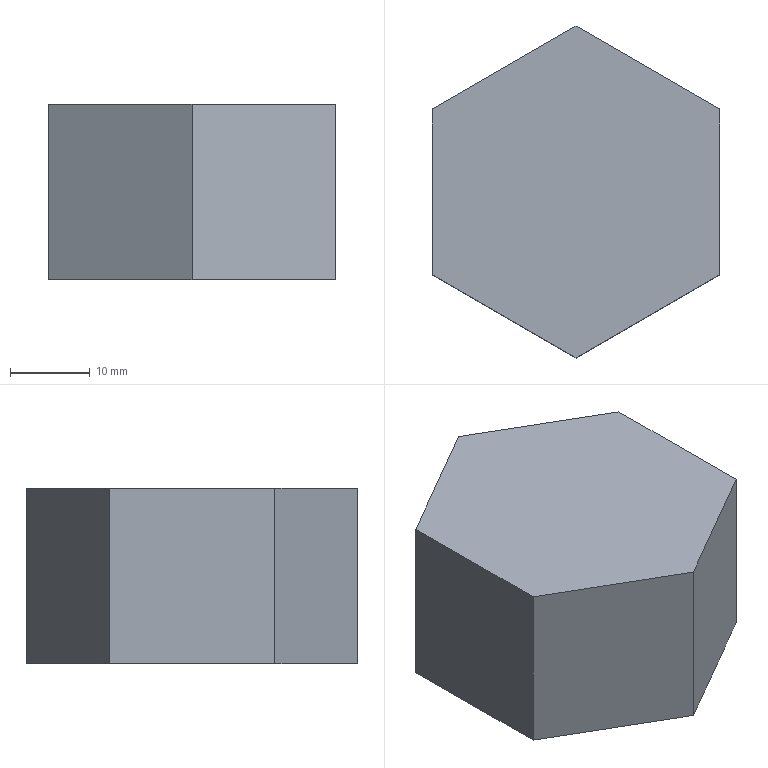Part | NX | features solid 2 | 1 solid | 8 faces | box 36 x 41.569 x 22 mm | volume 24692 mm3 | plane 8
STEP:
#1=CARTESIAN_POINT('',(670.5,-220.392,-53.));
#2=VERTEX_POINT('',#1);
#3=CARTESIAN_POINT('',(652.5,-230.785,-53.));
#4=VERTEX_POINT('',#3);
#5=CARTESIAN_POINT('',(670.5,-220.392,-53.));
#6=DIRECTION('',(-0.866,-0.5,0.));
#7=VECTOR('',#6,1000.);
#8=LINE('',#5,#7);
#9=EDGE_CURVE('',#2,#4,#8,.T.);
#10=ORIENTED_EDGE('',*,*,#9,.F.);
#11=CARTESIAN_POINT('',(670.5,-220.392,-31.));
#12=VERTEX_POINT('',#11);
#13=CARTESIAN_POINT('',(670.5,-220.392,-31.));
#14=DIRECTION('',(0.,0.,-1.));
#15=VECTOR('',#14,1000.);
#16=LINE('',#13,#15);
#17=EDGE_CURVE('',#12,#2,#16,.T.);
#18=ORIENTED_EDGE('',*,*,#17,.F.);
#19=CARTESIAN_POINT('',(652.5,-230.785,-31.));
#20=VERTEX_POINT('',#19);
#21=CARTESIAN_POINT('',(670.5,-220.392,-31.));
#22=DIRECTION('',(-0.866,-0.5,0.));
#23=VECTOR('',#22,1000.);
#24=LINE('',#21,#23);
#25=EDGE_CURVE('',#12,#20,#24,.T.);
#26=ORIENTED_EDGE('',*,*,#25,.T.);
#27=CARTESIAN_POINT('',(652.5,-230.785,-31.));
#28=DIRECTION('',(0.,0.,-1.));
#29=VECTOR('',#28,1000.);
#30=LINE('',#27,#29);
#31=EDGE_CURVE('',#20,#4,#30,.T.);
#32=ORIENTED_EDGE('',*,*,#31,.T.);
#33=EDGE_LOOP('',(#10,#18,#26,#32));
#34=FACE_BOUND('',#33,.T.);
#35=CARTESIAN_POINT('',(670.5,-220.392,-31.));
#36=DIRECTION('',(-0.5,0.866,0.));
#37=DIRECTION('',(0.866,0.5,0.));
#38=AXIS2_PLACEMENT_3D('',#35,#36,#37);
#39=PLANE('',#38);
#40=ADVANCED_FACE('',(#34),#39,.F.);
#41=CARTESIAN_POINT('',(634.5,-220.392,-53.));
#42=VERTEX_POINT('',#41);
#43=CARTESIAN_POINT('',(652.5,-230.785,-53.));
#44=DIRECTION('',(-0.866,0.5,0.));
#45=VECTOR('',#44,1000.);
#46=LINE('',#43,#45);
#47=EDGE_CURVE('',#4,#42,#46,.T.);
#48=ORIENTED_EDGE('',*,*,#47,.F.);
#49=ORIENTED_EDGE('',*,*,#31,.F.);
#50=CARTESIAN_POINT('',(634.5,-220.392,-31.));
#51=VERTEX_POINT('',#50);
#52=CARTESIAN_POINT('',(652.5,-230.785,-31.));
#53=DIRECTION('',(-0.866,0.5,0.));
#54=VECTOR('',#53,1000.);
#55=LINE('',#52,#54);
#56=EDGE_CURVE('',#20,#51,#55,.T.);
#57=ORIENTED_EDGE('',*,*,#56,.T.);
#58=CARTESIAN_POINT('',(634.5,-220.392,-31.));
#59=DIRECTION('',(0.,0.,-1.));
#60=VECTOR('',#59,1000.);
#61=LINE('',#58,#60);
#62=EDGE_CURVE('',#51,#42,#61,.T.);
#63=ORIENTED_EDGE('',*,*,#62,.T.);
#64=EDGE_LOOP('',(#48,#49,#57,#63));
#65=FACE_BOUND('',#64,.T.);
#66=CARTESIAN_POINT('',(652.5,-230.785,-31.));
#67=DIRECTION('',(0.5,0.866,0.));
#68=DIRECTION('',(0.866,-0.5,0.));
#69=AXIS2_PLACEMENT_3D('',#66,#67,#68);
#70=PLANE('',#69);
#71=ADVANCED_FACE('',(#65),#70,.F.);
#72=CARTESIAN_POINT('',(634.5,-199.608,-53.));
#73=VERTEX_POINT('',#72);
#74=CARTESIAN_POINT('',(634.5,-220.392,-53.));
#75=DIRECTION('',(0.,1.,0.));
#76=VECTOR('',#75,1000.);
#77=LINE('',#74,#76);
#78=EDGE_CURVE('',#42,#73,#77,.T.);
#79=ORIENTED_EDGE('',*,*,#78,.F.);
#80=ORIENTED_EDGE('',*,*,#62,.F.);
#81=CARTESIAN_POINT('',(634.5,-199.608,-31.));
#82=VERTEX_POINT('',#81);
#83=CARTESIAN_POINT('',(634.5,-220.392,-31.));
#84=DIRECTION('',(0.,1.,0.));
#85=VECTOR('',#84,1000.);
#86=LINE('',#83,#85);
#87=EDGE_CURVE('',#51,#82,#86,.T.);
#88=ORIENTED_EDGE('',*,*,#87,.T.);
#89=CARTESIAN_POINT('',(634.5,-199.608,-31.));
#90=DIRECTION('',(0.,0.,-1.));
#91=VECTOR('',#90,1000.);
#92=LINE('',#89,#91);
#93=EDGE_CURVE('',#82,#73,#92,.T.);
#94=ORIENTED_EDGE('',*,*,#93,.T.);
#95=EDGE_LOOP('',(#79,#80,#88,#94));
#96=FACE_BOUND('',#95,.T.);
#97=CARTESIAN_POINT('',(634.5,-220.392,-31.));
#98=DIRECTION('',(1.,0.,0.));
#99=DIRECTION('',(0.,-1.,0.));
#100=AXIS2_PLACEMENT_3D('',#97,#98,#99);
#101=PLANE('',#100);
#102=ADVANCED_FACE('',(#96),#101,.F.);
#103=CARTESIAN_POINT('',(652.5,-189.215,-53.));
#104=VERTEX_POINT('',#103);
#105=CARTESIAN_POINT('',(634.5,-199.608,-53.));
#106=DIRECTION('',(0.866,0.5,0.));
#107=VECTOR('',#106,1000.);
#108=LINE('',#105,#107);
#109=EDGE_CURVE('',#73,#104,#108,.T.);
#110=ORIENTED_EDGE('',*,*,#109,.F.);
#111=ORIENTED_EDGE('',*,*,#93,.F.);
#112=CARTESIAN_POINT('',(652.5,-189.215,-31.));
#113=VERTEX_POINT('',#112);
#114=CARTESIAN_POINT('',(634.5,-199.608,-31.));
#115=DIRECTION('',(0.866,0.5,0.));
#116=VECTOR('',#115,1000.);
#117=LINE('',#114,#116);
#118=EDGE_CURVE('',#82,#113,#117,.T.);
#119=ORIENTED_EDGE('',*,*,#118,.T.);
#120=CARTESIAN_POINT('',(652.5,-189.215,-31.));
#121=DIRECTION('',(0.,0.,-1.));
#122=VECTOR('',#121,1000.);
#123=LINE('',#120,#122);
#124=EDGE_CURVE('',#113,#104,#123,.T.);
#125=ORIENTED_EDGE('',*,*,#124,.T.);
#126=EDGE_LOOP('',(#110,#111,#119,#125));
#127=FACE_BOUND('',#126,.T.);
#128=CARTESIAN_POINT('',(634.5,-199.608,-31.));
#129=DIRECTION('',(0.5,-0.866,0.));
#130=DIRECTION('',(-0.866,-0.5,0.));
#131=AXIS2_PLACEMENT_3D('',#128,#129,#130);
#132=PLANE('',#131);
#133=ADVANCED_FACE('',(#127),#132,.F.);
#134=CARTESIAN_POINT('',(670.5,-199.608,-53.));
#135=VERTEX_POINT('',#134);
#136=CARTESIAN_POINT('',(652.5,-189.215,-53.));
#137=DIRECTION('',(0.866,-0.5,0.));
#138=VECTOR('',#137,1000.);
#139=LINE('',#136,#138);
#140=EDGE_CURVE('',#104,#135,#139,.T.);
#141=ORIENTED_EDGE('',*,*,#140,.F.);
#142=ORIENTED_EDGE('',*,*,#124,.F.);
#143=CARTESIAN_POINT('',(670.5,-199.608,-31.));
#144=VERTEX_POINT('',#143);
#145=CARTESIAN_POINT('',(652.5,-189.215,-31.));
#146=DIRECTION('',(0.866,-0.5,0.));
#147=VECTOR('',#146,1000.);
#148=LINE('',#145,#147);
#149=EDGE_CURVE('',#113,#144,#148,.T.);
#150=ORIENTED_EDGE('',*,*,#149,.T.);
#151=CARTESIAN_POINT('',(670.5,-199.608,-31.));
#152=DIRECTION('',(0.,0.,-1.));
#153=VECTOR('',#152,1000.);
#154=LINE('',#151,#153);
#155=EDGE_CURVE('',#144,#135,#154,.T.);
#156=ORIENTED_EDGE('',*,*,#155,.T.);
#157=EDGE_LOOP('',(#141,#142,#150,#156));
#158=FACE_BOUND('',#157,.T.);
#159=CARTESIAN_POINT('',(652.5,-189.215,-31.));
#160=DIRECTION('',(-0.5,-0.866,0.));
#161=DIRECTION('',(-0.866,0.5,0.));
#162=AXIS2_PLACEMENT_3D('',#159,#160,#161);
#163=PLANE('',#162);
#164=ADVANCED_FACE('',(#158),#163,.F.);
#165=CARTESIAN_POINT('',(670.5,-199.608,-53.));
#166=DIRECTION('',(0.,-1.,0.));
#167=VECTOR('',#166,1000.);
#168=LINE('',#165,#167);
#169=EDGE_CURVE('',#135,#2,#168,.T.);
#170=ORIENTED_EDGE('',*,*,#169,.F.);
#171=ORIENTED_EDGE('',*,*,#155,.F.);
#172=CARTESIAN_POINT('',(670.5,-199.608,-31.));
#173=DIRECTION('',(0.,-1.,0.));
#174=VECTOR('',#173,1000.);
#175=LINE('',#172,#174);
#176=EDGE_CURVE('',#144,#12,#175,.T.);
#177=ORIENTED_EDGE('',*,*,#176,.T.);
#178=ORIENTED_EDGE('',*,*,#17,.T.);
#179=EDGE_LOOP('',(#170,#171,#177,#178));
#180=FACE_BOUND('',#179,.T.);
#181=CARTESIAN_POINT('',(670.5,-199.608,-31.));
#182=DIRECTION('',(-1.,0.,0.));
#183=DIRECTION('',(0.,1.,0.));
#184=AXIS2_PLACEMENT_3D('',#181,#182,#183);
#185=PLANE('',#184);
#186=ADVANCED_FACE('',(#180),#185,.F.);
#187=ORIENTED_EDGE('',*,*,#25,.F.);
#188=ORIENTED_EDGE('',*,*,#176,.F.);
#189=ORIENTED_EDGE('',*,*,#149,.F.);
#190=ORIENTED_EDGE('',*,*,#118,.F.);
#191=ORIENTED_EDGE('',*,*,#87,.F.);
#192=ORIENTED_EDGE('',*,*,#56,.F.);
#193=EDGE_LOOP('',(#187,#188,#189,#190,#191,#192));
#194=FACE_BOUND('',#193,.T.);
#195=CARTESIAN_POINT('',(634.5,-241.177,-31.));
#196=DIRECTION('',(0.,0.,1.));
#197=DIRECTION('',(0.,1.,0.));
#198=AXIS2_PLACEMENT_3D('',#195,#196,#197);
#199=PLANE('',#198);
#200=ADVANCED_FACE('',(#194),#199,.T.);
#201=ORIENTED_EDGE('',*,*,#9,.T.);
#202=ORIENTED_EDGE('',*,*,#47,.T.);
#203=ORIENTED_EDGE('',*,*,#78,.T.);
#204=ORIENTED_EDGE('',*,*,#109,.T.);
#205=ORIENTED_EDGE('',*,*,#140,.T.);
#206=ORIENTED_EDGE('',*,*,#169,.T.);
#207=EDGE_LOOP('',(#201,#202,#203,#204,#205,#206));
#208=FACE_BOUND('',#207,.T.);
#209=CARTESIAN_POINT('',(634.5,-241.177,-53.));
#210=DIRECTION('',(0.,0.,1.));
#211=DIRECTION('',(0.,1.,0.));
#212=AXIS2_PLACEMENT_3D('',#209,#210,#211);
#213=PLANE('',#212);
#214=ADVANCED_FACE('',(#208),#213,.F.);
#215=CLOSED_SHELL('',(#40,#71,#102,#133,#164,#186,#200,#214));
#216=MANIFOLD_SOLID_BREP('',#215);
#217=(LENGTH_UNIT()NAMED_UNIT(*)SI_UNIT(.MILLI.,.METRE.));
#218=UNCERTAINTY_MEASURE_WITH_UNIT(LENGTH_MEASURE(0.00001),#217,'','');
#219=(NAMED_UNIT(*)PLANE_ANGLE_UNIT()SI_UNIT($,.RADIAN.));
#220=(NAMED_UNIT(*)SI_UNIT($,.STERADIAN.)SOLID_ANGLE_UNIT());
#221=(GEOMETRIC_REPRESENTATION_CONTEXT(3)GLOBAL_UNCERTAINTY_ASSIGNED_CONTEXT((#218))GLOBAL_UNIT_ASSIGNED_CONTEXT((#217,#219,#220))REPRESENTATION_CONTEXT('',''));
#222=ADVANCED_BREP_SHAPE_REPRESENTATION('',(#216),#221);